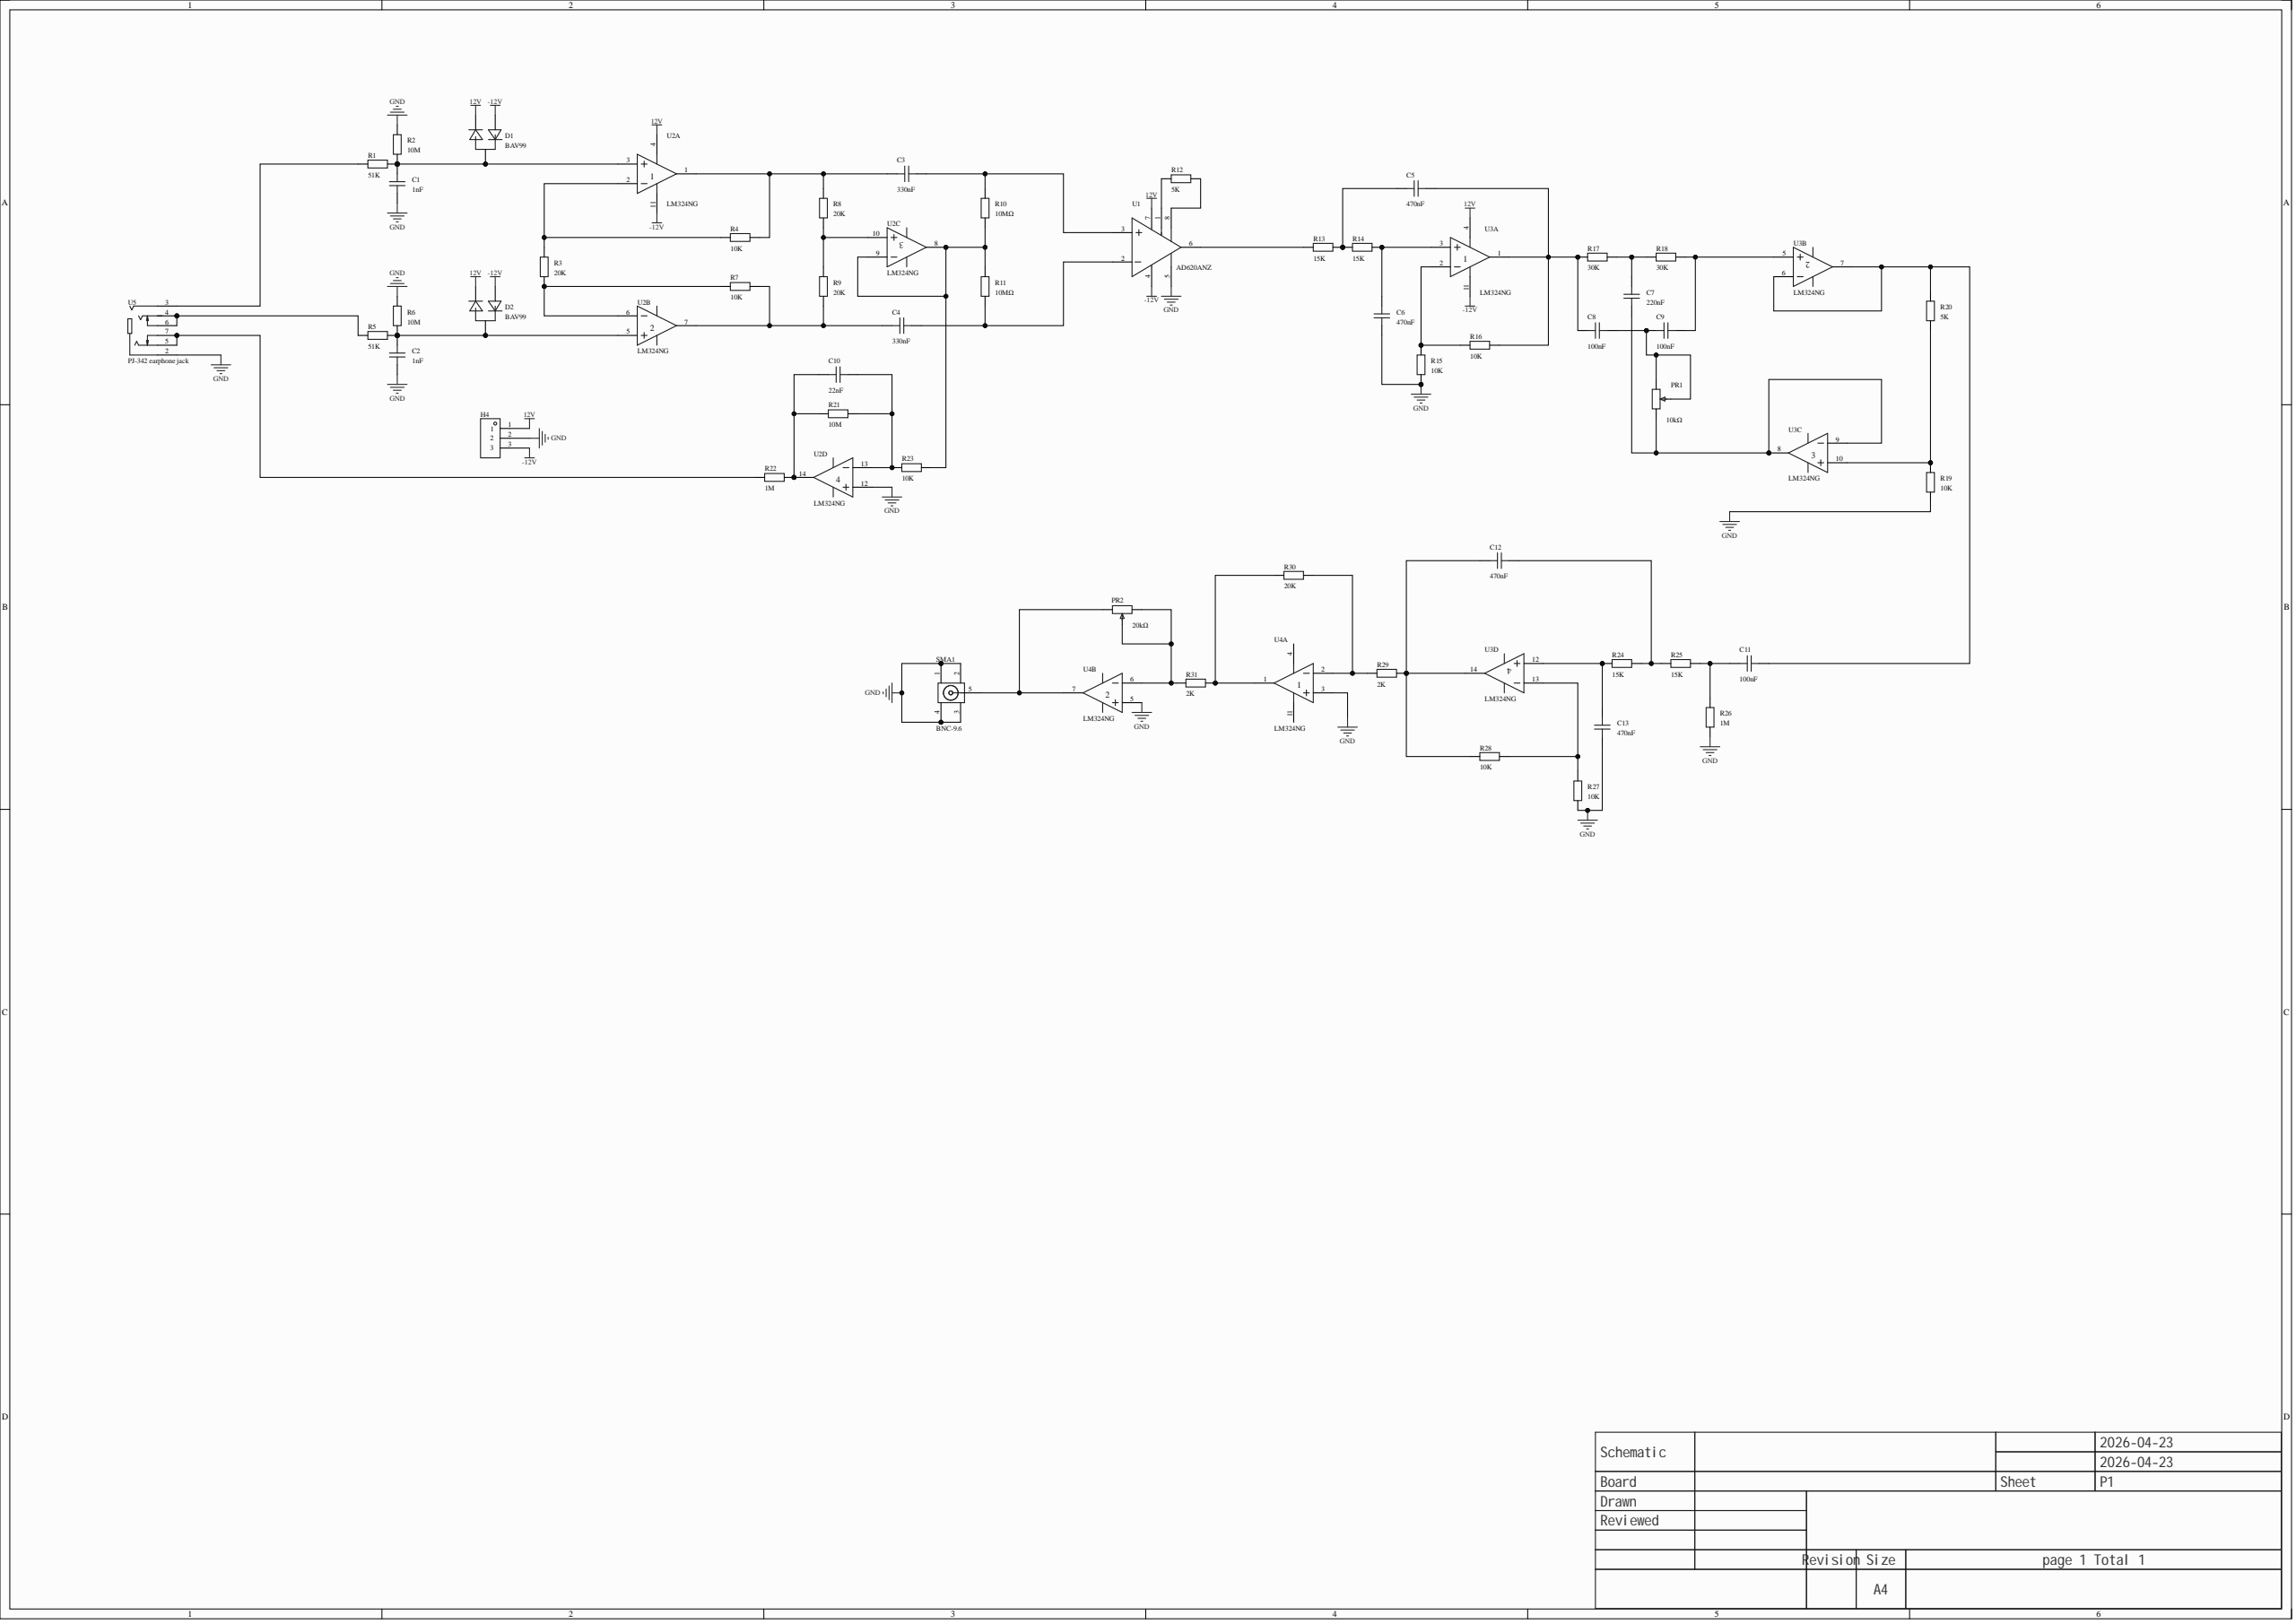Circuit board | Altium Designer | 55 parts | 40 nets
Bill of materials:
Comment,Description,Designator,Footprint,LibRef,Quantity
"1nF","","C1, C2","C0603","CAP_0603","2"
"330nF","","C3, C4","C0603","CAP_0603","2"
"470nF","","C5, C6, C12, C13","C0603","CAP_0603","4"
"220nF","","C7","C0603","CAP_0603","1"
"100nF","","C8, C9, C11","C0603","CAP_0603","3"
"22nF","","C10","C0603","CAP_0603","1"
"BAV99","Diode configuration: 1 pair in series; forward voltage (Vf): 1.25V; DC reverse voltage (Vr): 75V; rectified current: 215mA; reverse recovery time (Trr): 4ns;","D1, D2","SOT-23-3_L2.9-W1.3-P1.90-LS2.4-BR","BAV99_C458983","2"
"","","H4","HDR-TH_3P-P2.54-V-M","HDR-M_2.54_1x3P","1"
"10kΩ","","PR1","R_3296","R_3296","1"
"20kΩ","","PR2","R_3296","R_3296","1"
"51K","","R1, R5","R0603","Res_0603","2"
"10M","","R2, R6, R21","R0603","Res_0603","3"
"20K","","R3, R8, R9, R30","R0603","Res_0603","4"
"10K","","R4, R7, R15, R16, R19, R23, R27, R28","R0603","Res_0603","8"
"10MΩ","","R10, R11","R0603","Res_0603","2"
"5K","","R12, R20","R0603","Res_0603","2"
"15K","","R13, R14, R24, R25","R0603","Res_0603","4"
"30K","","R17, R18","R0603","Res_0603","2"
"1M","","R22, R26","R0603","Res_0603","2"
"2K","","R29, R31","R0603","Res_0603","2"
"BNC-9.6","","SMA1","SMA-TH_5P_BNC-9.6","BNC-9.6","1"
"AD620ANZ","Amplifiers: single; common-mode rejection ratio (CMRR): 100dB; input bias current (Ib): 500pA; input offset voltage (Vos): 30uV; gain-bandwidth product (GBP): -; slew rate (SR): 0.75V/us; bandwidth (-3dB): 120kHz;","U1","DIP-8_L9.3-W6.4-P2.54-LS7.6-BL","AD620ANZ","1"
"LM324NG","Amplifiers: 4; rail-to-rail: -; gain-bandwidth product (GBW): -; input offset voltage (Vos): 5mV; slew rate (SR): 600V/ms; input bias current (Ib): 300nA;","U2, U3, U4","PDIP-14_L19.7-W6.6-P2.54-LS8.3-BL","LM324NG","3"
"PJ-342 earphone jack","","U5","AUDIO-SMD_PJ-342_C9900012319","PJ-342耳机座","1"
Netlist (Protel format):
[
C1
C0603
1nF



]
[
C2
C0603
1nF



]
[
C3
C0603
330nF



]
[
C4
C0603
330nF



]
[
C5
C0603
470nF



]
[
C6
C0603
470nF



]
[
C7
C0603
220nF



]
[
C8
C0603
100nF



]
[
C9
C0603
100nF



]
[
C10
C0603
22nF



]
[
C11
C0603
100nF



]
[
C12
C0603
470nF



]
[
C13
C0603
470nF



]
[
D1
SOT-23-3_L2.9-W1.3-P1.90-LS2.4-BR
BAV99



]
[
D2
SOT-23-3_L2.9-W1.3-P1.90-LS2.4-BR
BAV99



]
[
H4
HDR-TH_3P-P2.54-V-M




]
[
PR1
R_3296
10kΩ



]
[
PR2
R_3296
20kΩ



]
[
R1
R0603
51K



]
[
R2
R0603
10M



]
[
R3
R0603
20K



]
[
R4
R0603
10K



]
[
R5
R0603
51K



]
[
R6
R0603
10M



]
[
R7
R0603
10K



]
[
R8
R0603
20K



]
[
R9
R0603
20K



]
[
R10
R0603
10MΩ



]
[
R11
R0603
10MΩ



]
[
R12
R0603
5K



]
[
R13
R0603
15K



]
[
R14
R0603
15K



]
[
R15
R0603
10K



]
[
R16
R0603
10K



]
[
R17
R0603
30K



]
[
R18
R0603
30K



]
[
R19
R0603
10K



]
[
R20
R0603
5K



]
[
R21
R0603
10M



]
[
R22
R0603
1M



]
[
R23
R0603
10K



]
[
R24
R0603
15K



]
[
R25
R0603
15K



]
[
R26
R0603
1M



]
[
R27
R0603
10K



]
[
R28
R0603
10K



]
[
R29
R0603
2K



]
[
R30
R0603
20K



]
[
R31
R0603
2K



]
[
SMA1
SMA-TH_5P_BNC-9.6
BNC-9.6



]
[
U1
DIP-8_L9.3-W6.4-P2.54-LS7.6-BL
AD620ANZ



]
[
U2
PDIP-14_L19.7-W6.6-P2.54-LS8.3-BL
LM324NG



]
[
U3
PDIP-14_L19.7-W6.6-P2.54-LS8.3-BL
LM324NG



]
[
U4
PDIP-14_L19.7-W6.6-P2.54-LS8.3-BL
LM324NG



]
[
U5
AUDIO-SMD_PJ-342_C9900012319
PJ-342 earphone jack



]
(
NetR30_1
R30-1
R31-2
U4-1
)
(
NetR29_1
R29-1
R30-2
U4-2
)
(
NetR27_2
R27-2
R28-1
U3-13
)
(
NetR22_1
R22-1
U5-5
U5-7
)
(
NetR19_2
R19-2
R20-1
U3-10
)
(
NetR15_2
R15-2
R16-2
U3-2
)
(
NetR13_1
R13-1
U1-6
)
(
NetR12_2
R12-2
U1-8
)
(
NetR12_1
R12-1
U1-1
)
(
NetR10_1
R10-1
R11-2
R23-2
U2-8
U2-9
)
(
NetR8_1
R8-1
R9-2
U2-10
)
(
NetR5_1
R5-1
U5-4
U5-6
)
(
NetR3_2
R3-2
R4-2
U2-2
)
(
NetR3_1
R3-1
R7-2
U2-6
)
(
NetR1_1
R1-1
U5-3
)
(
NetPR2_2
PR2-2
PR2-3
R31-1
U4-6
)
(
NetPR2_1
PR2-1
SMA1-5
U4-7
)
(
NetC13_2
C13-2
R24-1
U3-12
)
(
NetC12_2
C12-2
R24-2
R25-1
)
(
NetC12_1
C12-1
R28-2
R29-2
U3-14
)
(
NetC11_2
C11-2
R20-2
U3-6
U3-7
)
(
NetC11_1
C11-1
R25-2
R26-2
)
(
NetC10_2
C10-2
R21-2
R23-1
U2-13
)
(
NetC10_1
C10-1
R21-1
R22-2
U2-14
)
(
NetC9_1
C9-1
R18-2
U3-5
)
(
NetC8_1
C8-1
C9-2
PR1-2
PR1-3
)
(
NetC7_2
C7-2
R17-2
R18-1
)
(
NetC7_1
C7-1
PR1-1
U3-8
U3-9
)
(
NetC6_2
C6-2
R14-2
U3-3
)
(
NetC5_2
C5-2
C8-2
R16-1
R17-1
U3-1
)
(
NetC5_1
C5-1
R13-2
R14-1
)
(
NetC4_2
C4-2
R11-1
U1-2
)
(
NetC4_1
C4-1
R7-1
R9-1
U2-7
)
(
NetC3_2
C3-2
R10-2
U1-3
)
(
NetC3_1
C3-1
R4-1
R8-2
U2-1
)
(
NetC2_2
C2-2
D2-3
R5-2
R6-1
U2-5
)
(
NetC1_2
C1-2
D1-3
R1-2
R2-1
U2-3
)
(
GND
C1-1
C2-1
C6-1
C13-1
H4-2
R2-2
R6-2
R15-1
R19-1
R26-1
R27-1
SMA1-1
SMA1-2
SMA1-3
SMA1-4
U1-5
U2-12
U4-3
U4-5
U5-2
)
(
-12V
D1-1
D2-1
H4-3
U1-4
U2-11
U3-11
)
(
12V
D1-2
D2-2
H4-1
U1-7
U2-4
U3-4
)